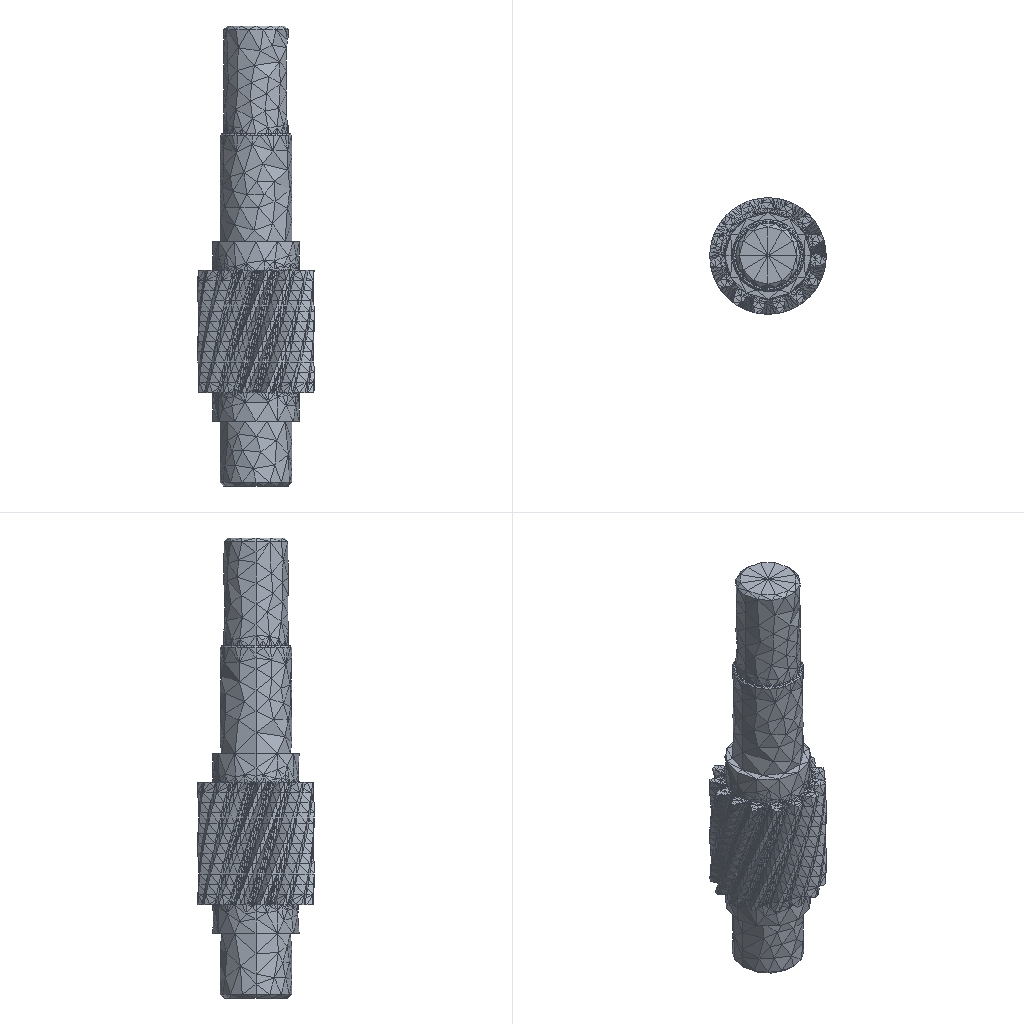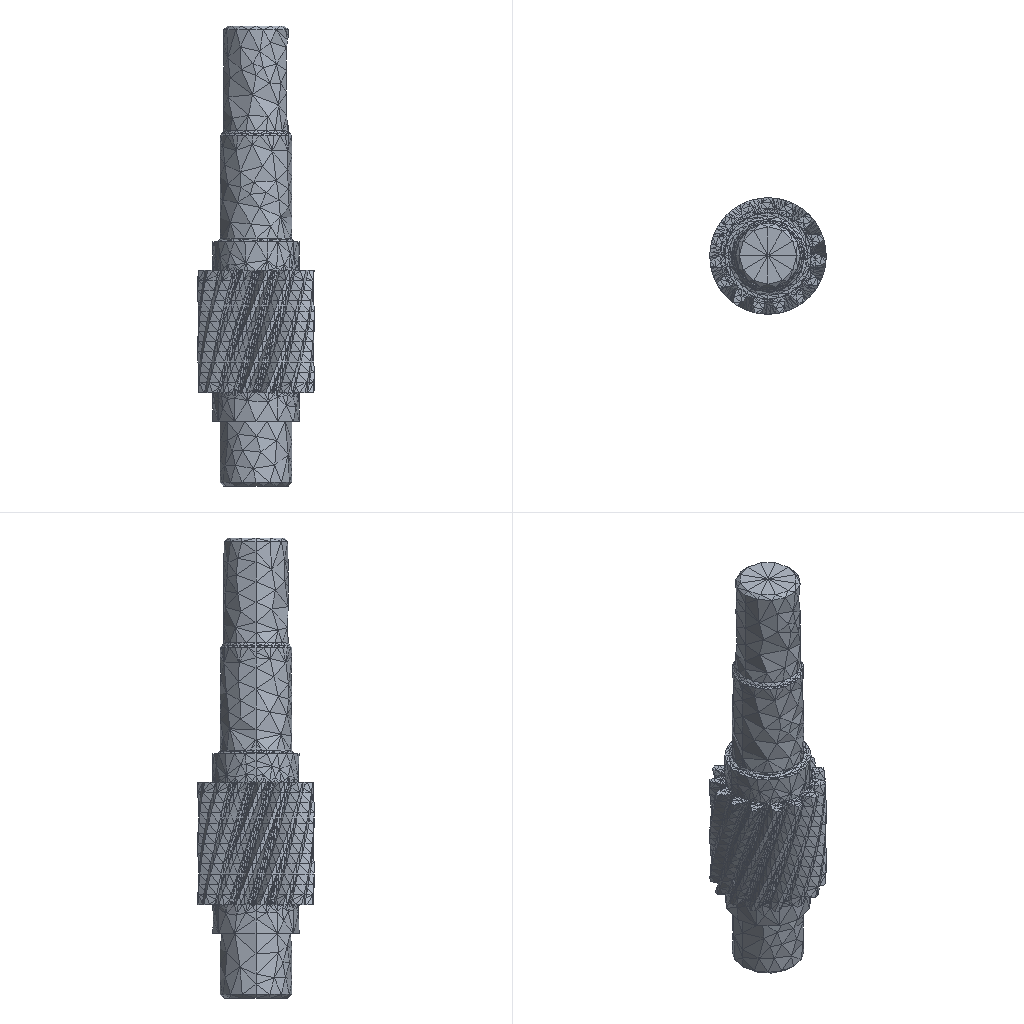Simulation study | ansys workbench
Set-up summary:
category,name,step,type,value,unit,region
solver,ansys_mapdl
solver,version,,,22.1
solver,version,,,22.1
solver,version,,,22.1
solver,version,,,22.1
solver,version,,,22.1
units,MPA,,stated
analysis,deck1,,modal,modal
load_step,requested,,,2
analysis,nlgeom,,,False
mesh,nodes,,,0
mesh,elements,,,0
load,load commands in deck,,count,0
bc,support commands in deck,,count,0
analysis,deck2,,static,static
load_step,requested,,,1
analysis,nlgeom,,,False
mesh,nodes,,,25171
mesh,elements,,,15253
element_type,ANSYS 187 (type 1),,solid,14648
element_type,ANSYS 174 (type 2),,contact,605
element_type,ANSYS 170 (type 3),,target,0
load,load commands in deck,,count,3
bc,support commands in deck,,count,1
named_set,_FIXEDSU,,component
analysis,deck3,,static,static
load_step,requested,,,1
analysis,nlgeom,,,False
mesh,nodes,,,25154
mesh,elements,,,15504
element_type,ANSYS 187 (type 1),,solid,14621
element_type,ANSYS 174 (type 2),,contact,883
element_type,ANSYS 170 (type 3),,target,0
load,load commands in deck,,count,3
bc,support commands in deck,,count,1
named_set,_CM29_FIXEDSU,,component
named_set,_FIXEDSU,,component
material,1,,in results
material,1,,in results
material,1,,in results
material,1,,in results
material,1,,in results
check,setup vs results,,match,results also hold 0 node(s) and 1 element(s) the deck makes with ['EN']; those were not compared; 1 node(s) the solver created internally for pilot nodes (solve.out) are in the results only
check,setup vs results,,match,results also hold 0 node(s) and 1 element(s) the deck makes with ['EN']; those were not compared; 1 node(s) the solver created internally for pilot nodes (solve.out) are in the results only
check,setup vs results,,match,results also hold 0 node(s) and 1 element(s) the deck makes with ['EN']; those were not compared; 1 node(s) the solver created internally for pilot nodes (solve.out) are in the results only
Results summary:
result,analysis,,,modal
result,last_loadstep,,,1
result,primary field,,,displacement
result,analysis,,,static
result,last_loadstep,,,1
result,primary field,,,displacement
result,reaction total,1,FX,5e-06,N
result,reaction total,1,FY,2e-06,N
result,reaction total,1,FZ,-5e-06,N
result,mass,,,0.0004,"NMM: mm, ton, N, s, mV, mA, degC"
result,analysis,,,static
result,last_loadstep,,,1
result,primary field,,,displacement
result,reaction total,1,FX,-16.475,N
result,reaction total,1,FY,-5781.404,N
result,reaction total,1,FZ,-193.127,N
result,mass,,,0.000185,"NMM: mm, ton, N, s, mV, mA, degC"
result,analysis,,,static
result,last_loadstep,,,1
result,primary field,,,displacement
result,reaction total,1,FX,16.475,N
result,reaction total,1,FY,5781.404,N
result,reaction total,1,FZ,193.127,N
result,mass,,,0.000215,"NMM: mm, ton, N, s, mV, mA, degC"
result,analysis,,,static
result,last_loadstep,,,1
result,primary field,,,displacement
result,reaction total,1,FX,-4e-06,N
result,reaction total,1,FY,-4e-06,N
result,reaction total,1,FZ,0.0,N
result,mass,,,0.0004,"NMM: mm, ton, N, s, mV, mA, degC"